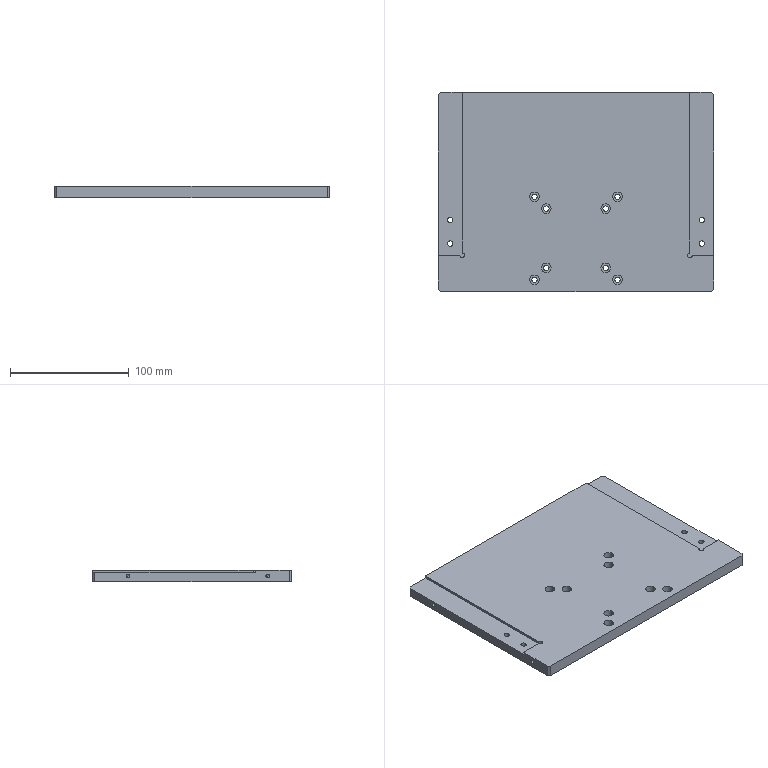Part | SolidWorks | features BaseBody 1 | 1 solid | 111 faces | box 232 x 168 x 10 mm | volume 373351 mm3 | cylinder 67 | plane 28 | cone 16 | commonest cylinder face diameters 4.5 x24 8 x24 3.3 x16 4 x3